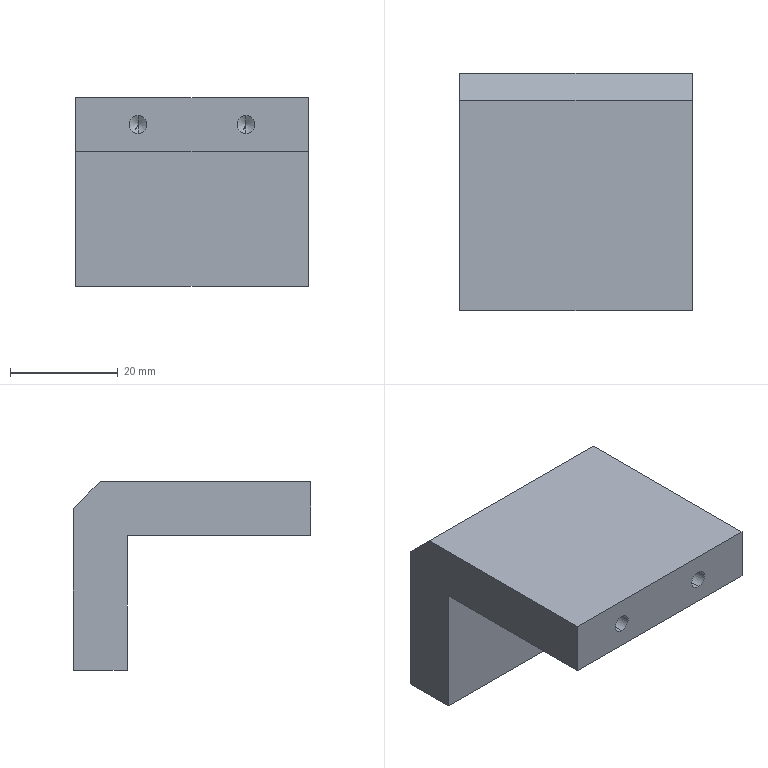Part | SolidWorks | features HoleWzd 2, Chamfer 1, Extrusion 1, ICE 1 | 1 solid | 25 faces | box 43 x 44 x 35 mm | volume 28591 mm3 | plane 9 | cylinder 8 | cone 8 | commonest cylinder face diameters 3.3 x8
STEP:
#1=CARTESIAN_POINT('',(-10.,-6.5,14.15));
#2=VERTEX_POINT('',#1);
#3=CARTESIAN_POINT('',(-10.,-6.5,10.85));
#4=VERTEX_POINT('',#3);
#5=CARTESIAN_POINT('',(-10.,-6.5,12.5));
#6=DIRECTION('',(0.,-1.,0.));
#7=DIRECTION('',(0.,0.,-1.));
#8=AXIS2_PLACEMENT_3D('',#5,#6,#7);
#9=CIRCLE('',#8,1.65);
#10=EDGE_CURVE('',#2,#4,#9,.T.);
#11=ORIENTED_EDGE('',*,*,#10,.F.);
#12=CARTESIAN_POINT('',(-10.,-22.,14.15));
#13=VERTEX_POINT('',#12);
#14=CARTESIAN_POINT('',(-10.,-22.,14.15));
#15=DIRECTION('',(0.,-1.,0.));
#16=VECTOR('',#15,1000.);
#17=LINE('',#14,#16);
#18=EDGE_CURVE('',#2,#13,#17,.T.);
#19=ORIENTED_EDGE('',*,*,#18,.T.);
#20=CARTESIAN_POINT('',(-10.,-22.,10.85));
#21=VERTEX_POINT('',#20);
#22=CARTESIAN_POINT('',(-10.,-22.,12.5));
#23=DIRECTION('',(0.,-1.,0.));
#24=DIRECTION('',(0.,0.,-1.));
#25=AXIS2_PLACEMENT_3D('',#22,#23,#24);
#26=CIRCLE('',#25,1.65);
#27=EDGE_CURVE('',#13,#21,#26,.T.);
#28=ORIENTED_EDGE('',*,*,#27,.T.);
#29=CARTESIAN_POINT('',(-10.,-22.,10.85));
#30=DIRECTION('',(0.,-1.,0.));
#31=VECTOR('',#30,1000.);
#32=LINE('',#29,#31);
#33=EDGE_CURVE('',#4,#21,#32,.T.);
#34=ORIENTED_EDGE('',*,*,#33,.F.);
#35=EDGE_LOOP('',(#11,#19,#28,#34));
#36=FACE_OUTER_BOUND('',#35,.T.);
#37=CARTESIAN_POINT('',(-10.,-22.,12.5));
#38=DIRECTION('',(0.,-1.,0.));
#39=DIRECTION('',(0.,0.,-1.));
#40=AXIS2_PLACEMENT_3D('',#37,#38,#39);
#41=CYLINDRICAL_SURFACE('',#40,1.65);
#42=ADVANCED_FACE('',(#36),#41,.F.);
#43=CARTESIAN_POINT('',(-10.,-5.509,12.5));
#44=VERTEX_POINT('',#43);
#45=CARTESIAN_POINT('',(-10.,-6.5,10.85));
#46=DIRECTION('',(0.,-0.515,-0.8572));
#47=VECTOR('',#46,1000.);
#48=LINE('',#45,#47);
#49=EDGE_CURVE('',#44,#4,#48,.T.);
#50=ORIENTED_EDGE('',*,*,#49,.F.);
#51=CARTESIAN_POINT('',(-10.,-6.5,14.15));
#52=DIRECTION('',(0.,-0.515,0.8572));
#53=VECTOR('',#52,1000.);
#54=LINE('',#51,#53);
#55=EDGE_CURVE('',#44,#2,#54,.T.);
#56=ORIENTED_EDGE('',*,*,#55,.T.);
#57=ORIENTED_EDGE('',*,*,#10,.T.);
#58=EDGE_LOOP('',(#50,#56,#57));
#59=FACE_OUTER_BOUND('',#58,.T.);
#60=CARTESIAN_POINT('',(-10.,-6.5,12.5));
#61=DIRECTION('',(0.,-1.,0.));
#62=DIRECTION('',(0.,0.,-1.));
#63=AXIS2_PLACEMENT_3D('',#60,#61,#62);
#64=CONICAL_SURFACE('',#63,1.65,1.03);
#65=ADVANCED_FACE('',(#59),#64,.F.);
#66=CARTESIAN_POINT('',(10.,-6.5,14.15));
#67=VERTEX_POINT('',#66);
#68=CARTESIAN_POINT('',(10.,-6.5,10.85));
#69=VERTEX_POINT('',#68);
#70=CARTESIAN_POINT('',(10.,-6.5,12.5));
#71=DIRECTION('',(0.,-1.,0.));
#72=DIRECTION('',(0.,0.,-1.));
#73=AXIS2_PLACEMENT_3D('',#70,#71,#72);
#74=CIRCLE('',#73,1.65);
#75=EDGE_CURVE('',#67,#69,#74,.T.);
#76=ORIENTED_EDGE('',*,*,#75,.F.);
#77=CARTESIAN_POINT('',(10.,-22.,14.15));
#78=VERTEX_POINT('',#77);
#79=CARTESIAN_POINT('',(10.,-22.,14.15));
#80=DIRECTION('',(0.,-1.,0.));
#81=VECTOR('',#80,1000.);
#82=LINE('',#79,#81);
#83=EDGE_CURVE('',#67,#78,#82,.T.);
#84=ORIENTED_EDGE('',*,*,#83,.T.);
#85=CARTESIAN_POINT('',(10.,-22.,10.85));
#86=VERTEX_POINT('',#85);
#87=CARTESIAN_POINT('',(10.,-22.,12.5));
#88=DIRECTION('',(0.,-1.,0.));
#89=DIRECTION('',(0.,0.,-1.));
#90=AXIS2_PLACEMENT_3D('',#87,#88,#89);
#91=CIRCLE('',#90,1.65);
#92=EDGE_CURVE('',#78,#86,#91,.T.);
#93=ORIENTED_EDGE('',*,*,#92,.T.);
#94=CARTESIAN_POINT('',(10.,-22.,10.85));
#95=DIRECTION('',(0.,-1.,0.));
#96=VECTOR('',#95,1000.);
#97=LINE('',#94,#96);
#98=EDGE_CURVE('',#69,#86,#97,.T.);
#99=ORIENTED_EDGE('',*,*,#98,.F.);
#100=EDGE_LOOP('',(#76,#84,#93,#99));
#101=FACE_OUTER_BOUND('',#100,.T.);
#102=CARTESIAN_POINT('',(10.,-22.,12.5));
#103=DIRECTION('',(0.,-1.,0.));
#104=DIRECTION('',(0.,0.,-1.));
#105=AXIS2_PLACEMENT_3D('',#102,#103,#104);
#106=CYLINDRICAL_SURFACE('',#105,1.65);
#107=ADVANCED_FACE('',(#101),#106,.F.);
#108=CARTESIAN_POINT('',(10.,-5.509,12.5));
#109=VERTEX_POINT('',#108);
#110=CARTESIAN_POINT('',(10.,-6.5,10.85));
#111=DIRECTION('',(0.,-0.515,-0.8572));
#112=VECTOR('',#111,1000.);
#113=LINE('',#110,#112);
#114=EDGE_CURVE('',#109,#69,#113,.T.);
#115=ORIENTED_EDGE('',*,*,#114,.F.);
#116=CARTESIAN_POINT('',(10.,-6.5,14.15));
#117=DIRECTION('',(0.,-0.515,0.8572));
#118=VECTOR('',#117,1000.);
#119=LINE('',#116,#118);
#120=EDGE_CURVE('',#109,#67,#119,.T.);
#121=ORIENTED_EDGE('',*,*,#120,.T.);
#122=ORIENTED_EDGE('',*,*,#75,.T.);
#123=EDGE_LOOP('',(#115,#121,#122));
#124=FACE_OUTER_BOUND('',#123,.T.);
#125=CARTESIAN_POINT('',(10.,-6.5,12.5));
#126=DIRECTION('',(0.,-1.,0.));
#127=DIRECTION('',(0.,0.,-1.));
#128=AXIS2_PLACEMENT_3D('',#125,#126,#127);
#129=CONICAL_SURFACE('',#128,1.65,1.03);
#130=ADVANCED_FACE('',(#124),#129,.F.);
#131=CARTESIAN_POINT('',(16.65,17.,-2.));
#132=VERTEX_POINT('',#131);
#133=CARTESIAN_POINT('',(13.35,17.,-2.));
#134=VERTEX_POINT('',#133);
#135=CARTESIAN_POINT('',(15.,17.,-2.));
#136=DIRECTION('',(0.,0.,-1.));
#137=DIRECTION('',(-1.,0.,0.));
#138=AXIS2_PLACEMENT_3D('',#135,#136,#137);
#139=CIRCLE('',#138,1.65);
#140=EDGE_CURVE('',#132,#134,#139,.T.);
#141=ORIENTED_EDGE('',*,*,#140,.F.);
#142=CARTESIAN_POINT('',(16.65,17.,-17.5));
#143=VERTEX_POINT('',#142);
#144=CARTESIAN_POINT('',(16.65,17.,-17.5));
#145=DIRECTION('',(0.,0.,-1.));
#146=VECTOR('',#145,1000.);
#147=LINE('',#144,#146);
#148=EDGE_CURVE('',#132,#143,#147,.T.);
#149=ORIENTED_EDGE('',*,*,#148,.T.);
#150=CARTESIAN_POINT('',(13.35,17.,-17.5));
#151=VERTEX_POINT('',#150);
#152=CARTESIAN_POINT('',(15.,17.,-17.5));
#153=DIRECTION('',(0.,0.,-1.));
#154=DIRECTION('',(-1.,0.,0.));
#155=AXIS2_PLACEMENT_3D('',#152,#153,#154);
#156=CIRCLE('',#155,1.65);
#157=EDGE_CURVE('',#143,#151,#156,.T.);
#158=ORIENTED_EDGE('',*,*,#157,.T.);
#159=CARTESIAN_POINT('',(13.35,17.,-17.5));
#160=DIRECTION('',(0.,0.,-1.));
#161=VECTOR('',#160,1000.);
#162=LINE('',#159,#161);
#163=EDGE_CURVE('',#134,#151,#162,.T.);
#164=ORIENTED_EDGE('',*,*,#163,.F.);
#165=EDGE_LOOP('',(#141,#149,#158,#164));
#166=FACE_OUTER_BOUND('',#165,.T.);
#167=CARTESIAN_POINT('',(15.,17.,-17.5));
#168=DIRECTION('',(0.,0.,-1.));
#169=DIRECTION('',(-1.,0.,0.));
#170=AXIS2_PLACEMENT_3D('',#167,#168,#169);
#171=CYLINDRICAL_SURFACE('',#170,1.65);
#172=ADVANCED_FACE('',(#166),#171,.F.);
#173=CARTESIAN_POINT('',(15.,17.,-1.009));
#174=VERTEX_POINT('',#173);
#175=CARTESIAN_POINT('',(13.35,17.,-2.));
#176=DIRECTION('',(-0.8572,0.,-0.515));
#177=VECTOR('',#176,1000.);
#178=LINE('',#175,#177);
#179=EDGE_CURVE('',#174,#134,#178,.T.);
#180=ORIENTED_EDGE('',*,*,#179,.F.);
#181=CARTESIAN_POINT('',(16.65,17.,-2.));
#182=DIRECTION('',(0.8572,0.,-0.515));
#183=VECTOR('',#182,1000.);
#184=LINE('',#181,#183);
#185=EDGE_CURVE('',#174,#132,#184,.T.);
#186=ORIENTED_EDGE('',*,*,#185,.T.);
#187=ORIENTED_EDGE('',*,*,#140,.T.);
#188=EDGE_LOOP('',(#180,#186,#187));
#189=FACE_OUTER_BOUND('',#188,.T.);
#190=CARTESIAN_POINT('',(15.,17.,-2.));
#191=DIRECTION('',(0.,0.,-1.));
#192=DIRECTION('',(-1.,0.,0.));
#193=AXIS2_PLACEMENT_3D('',#190,#191,#192);
#194=CONICAL_SURFACE('',#193,1.65,1.03);
#195=ADVANCED_FACE('',(#189),#194,.F.);
#196=CARTESIAN_POINT('',(-13.35,17.,-2.));
#197=VERTEX_POINT('',#196);
#198=CARTESIAN_POINT('',(-16.65,17.,-2.));
#199=VERTEX_POINT('',#198);
#200=CARTESIAN_POINT('',(-15.,17.,-2.));
#201=DIRECTION('',(0.,0.,-1.));
#202=DIRECTION('',(-1.,0.,0.));
#203=AXIS2_PLACEMENT_3D('',#200,#201,#202);
#204=CIRCLE('',#203,1.65);
#205=EDGE_CURVE('',#197,#199,#204,.T.);
#206=ORIENTED_EDGE('',*,*,#205,.F.);
#207=CARTESIAN_POINT('',(-13.35,17.,-17.5));
#208=VERTEX_POINT('',#207);
#209=CARTESIAN_POINT('',(-13.35,17.,-17.5));
#210=DIRECTION('',(0.,0.,-1.));
#211=VECTOR('',#210,1000.);
#212=LINE('',#209,#211);
#213=EDGE_CURVE('',#197,#208,#212,.T.);
#214=ORIENTED_EDGE('',*,*,#213,.T.);
#215=CARTESIAN_POINT('',(-16.65,17.,-17.5));
#216=VERTEX_POINT('',#215);
#217=CARTESIAN_POINT('',(-15.,17.,-17.5));
#218=DIRECTION('',(0.,0.,-1.));
#219=DIRECTION('',(-1.,0.,0.));
#220=AXIS2_PLACEMENT_3D('',#217,#218,#219);
#221=CIRCLE('',#220,1.65);
#222=EDGE_CURVE('',#208,#216,#221,.T.);
#223=ORIENTED_EDGE('',*,*,#222,.T.);
#224=CARTESIAN_POINT('',(-16.65,17.,-17.5));
#225=DIRECTION('',(0.,0.,-1.));
#226=VECTOR('',#225,1000.);
#227=LINE('',#224,#226);
#228=EDGE_CURVE('',#199,#216,#227,.T.);
#229=ORIENTED_EDGE('',*,*,#228,.F.);
#230=EDGE_LOOP('',(#206,#214,#223,#229));
#231=FACE_OUTER_BOUND('',#230,.T.);
#232=CARTESIAN_POINT('',(-15.,17.,-17.5));
#233=DIRECTION('',(0.,0.,-1.));
#234=DIRECTION('',(-1.,0.,0.));
#235=AXIS2_PLACEMENT_3D('',#232,#233,#234);
#236=CYLINDRICAL_SURFACE('',#235,1.65);
#237=ADVANCED_FACE('',(#231),#236,.F.);
#238=CARTESIAN_POINT('',(-15.,17.,-1.009));
#239=VERTEX_POINT('',#238);
#240=CARTESIAN_POINT('',(-16.65,17.,-2.));
#241=DIRECTION('',(-0.8572,0.,-0.515));
#242=VECTOR('',#241,1000.);
#243=LINE('',#240,#242);
#244=EDGE_CURVE('',#239,#199,#243,.T.);
#245=ORIENTED_EDGE('',*,*,#244,.F.);
#246=CARTESIAN_POINT('',(-13.35,17.,-2.));
#247=DIRECTION('',(0.8572,0.,-0.515));
#248=VECTOR('',#247,1000.);
#249=LINE('',#246,#248);
#250=EDGE_CURVE('',#239,#197,#249,.T.);
#251=ORIENTED_EDGE('',*,*,#250,.T.);
#252=ORIENTED_EDGE('',*,*,#205,.T.);
#253=EDGE_LOOP('',(#245,#251,#252));
#254=FACE_OUTER_BOUND('',#253,.T.);
#255=CARTESIAN_POINT('',(-15.,17.,-2.));
#256=DIRECTION('',(0.,0.,-1.));
#257=DIRECTION('',(-1.,0.,0.));
#258=AXIS2_PLACEMENT_3D('',#255,#256,#257);
#259=CONICAL_SURFACE('',#258,1.65,1.03);
#260=ADVANCED_FACE('',(#254),#259,.F.);
#261=CARTESIAN_POINT('',(21.5,22.,12.5));
#262=VERTEX_POINT('',#261);
#263=CARTESIAN_POINT('',(21.5,22.,-17.5));
#264=VERTEX_POINT('',#263);
#265=CARTESIAN_POINT('',(21.5,22.,17.5));
#266=DIRECTION('',(0.,0.,-1.));
#267=VECTOR('',#266,1000.);
#268=LINE('',#265,#267);
#269=EDGE_CURVE('',#262,#264,#268,.T.);
#270=ORIENTED_EDGE('',*,*,#269,.F.);
#271=CARTESIAN_POINT('',(21.5,17.,17.5));
#272=VERTEX_POINT('',#271);
#273=CARTESIAN_POINT('',(21.5,17.,17.5));
#274=DIRECTION('',(0.,-0.7071,0.7071));
#275=VECTOR('',#274,1000.);
#276=LINE('',#273,#275);
#277=EDGE_CURVE('',#262,#272,#276,.T.);
#278=ORIENTED_EDGE('',*,*,#277,.T.);
#279=CARTESIAN_POINT('',(21.5,-22.,17.5));
#280=VERTEX_POINT('',#279);
#281=CARTESIAN_POINT('',(21.5,22.,17.5));
#282=DIRECTION('',(0.,1.,0.));
#283=VECTOR('',#282,1000.);
#284=LINE('',#281,#283);
#285=EDGE_CURVE('',#280,#272,#284,.T.);
#286=ORIENTED_EDGE('',*,*,#285,.F.);
#287=CARTESIAN_POINT('',(21.5,-22.,7.5));
#288=VERTEX_POINT('',#287);
#289=CARTESIAN_POINT('',(21.5,-22.,17.5));
#290=DIRECTION('',(0.,0.,-1.));
#291=VECTOR('',#290,1000.);
#292=LINE('',#289,#291);
#293=EDGE_CURVE('',#280,#288,#292,.T.);
#294=ORIENTED_EDGE('',*,*,#293,.T.);
#295=CARTESIAN_POINT('',(21.5,12.,7.5));
#296=VERTEX_POINT('',#295);
#297=CARTESIAN_POINT('',(21.5,-56.,7.5));
#298=DIRECTION('',(0.,-1.,0.));
#299=VECTOR('',#298,1000.);
#300=LINE('',#297,#299);
#301=EDGE_CURVE('',#296,#288,#300,.T.);
#302=ORIENTED_EDGE('',*,*,#301,.F.);
#303=CARTESIAN_POINT('',(21.5,12.,-17.5));
#304=VERTEX_POINT('',#303);
#305=CARTESIAN_POINT('',(21.5,12.,-42.5));
#306=DIRECTION('',(0.,0.,1.));
#307=VECTOR('',#306,1000.);
#308=LINE('',#305,#307);
#309=EDGE_CURVE('',#304,#296,#308,.T.);
#310=ORIENTED_EDGE('',*,*,#309,.F.);
#311=CARTESIAN_POINT('',(21.5,22.,-17.5));
#312=DIRECTION('',(0.,1.,0.));
#313=VECTOR('',#312,1000.);
#314=LINE('',#311,#313);
#315=EDGE_CURVE('',#304,#264,#314,.T.);
#316=ORIENTED_EDGE('',*,*,#315,.T.);
#317=EDGE_LOOP('',(#270,#278,#286,#294,#302,#310,#316));
#318=FACE_OUTER_BOUND('',#317,.T.);
#319=CARTESIAN_POINT('',(21.5,22.,17.5));
#320=DIRECTION('',(-1.,0.,0.));
#321=DIRECTION('',(0.,-1.,0.));
#322=AXIS2_PLACEMENT_3D('',#319,#320,#321);
#323=PLANE('',#322);
#324=ADVANCED_FACE('',(#318),#323,.F.);
#325=CARTESIAN_POINT('',(-21.5,22.,12.5));
#326=VERTEX_POINT('',#325);
#327=CARTESIAN_POINT('',(-21.5,22.,-17.5));
#328=VERTEX_POINT('',#327);
#329=CARTESIAN_POINT('',(-21.5,22.,17.5));
#330=DIRECTION('',(0.,0.,-1.));
#331=VECTOR('',#330,1000.);
#332=LINE('',#329,#331);
#333=EDGE_CURVE('',#326,#328,#332,.T.);
#334=ORIENTED_EDGE('',*,*,#333,.F.);
#335=CARTESIAN_POINT('',(21.5,22.,12.5));
#336=DIRECTION('',(1.,0.,0.));
#337=VECTOR('',#336,1000.);
#338=LINE('',#335,#337);
#339=EDGE_CURVE('',#326,#262,#338,.T.);
#340=ORIENTED_EDGE('',*,*,#339,.T.);
#341=ORIENTED_EDGE('',*,*,#269,.T.);
#342=CARTESIAN_POINT('',(-21.5,22.,-17.5));
#343=DIRECTION('',(-1.,0.,0.));
#344=VECTOR('',#343,1000.);
#345=LINE('',#342,#344);
#346=EDGE_CURVE('',#264,#328,#345,.T.);
#347=ORIENTED_EDGE('',*,*,#346,.T.);
#348=EDGE_LOOP('',(#334,#340,#341,#347));
#349=FACE_OUTER_BOUND('',#348,.T.);
#350=CARTESIAN_POINT('',(-21.5,22.,17.5));
#351=DIRECTION('',(0.,-1.,0.));
#352=DIRECTION('',(0.,0.,-1.));
#353=AXIS2_PLACEMENT_3D('',#350,#351,#352);
#354=PLANE('',#353);
#355=ADVANCED_FACE('',(#349),#354,.F.);
#356=CARTESIAN_POINT('',(-21.5,17.,17.5));
#357=VERTEX_POINT('',#356);
#358=CARTESIAN_POINT('',(-21.5,-22.,17.5));
#359=VERTEX_POINT('',#358);
#360=CARTESIAN_POINT('',(-21.5,22.,17.5));
#361=DIRECTION('',(0.,-1.,0.));
#362=VECTOR('',#361,1000.);
#363=LINE('',#360,#362);
#364=EDGE_CURVE('',#357,#359,#363,.T.);
#365=ORIENTED_EDGE('',*,*,#364,.F.);
#366=CARTESIAN_POINT('',(-21.5,17.,17.5));
#367=DIRECTION('',(0.,0.7071,-0.7071));
#368=VECTOR('',#367,1000.);
#369=LINE('',#366,#368);
#370=EDGE_CURVE('',#357,#326,#369,.T.);
#371=ORIENTED_EDGE('',*,*,#370,.T.);
#372=ORIENTED_EDGE('',*,*,#333,.T.);
#373=CARTESIAN_POINT('',(-21.5,12.,-17.5));
#374=VERTEX_POINT('',#373);
#375=CARTESIAN_POINT('',(-21.5,22.,-17.5));
#376=DIRECTION('',(0.,-1.,0.));
#377=VECTOR('',#376,1000.);
#378=LINE('',#375,#377);
#379=EDGE_CURVE('',#328,#374,#378,.T.);
#380=ORIENTED_EDGE('',*,*,#379,.T.);
#381=CARTESIAN_POINT('',(-21.5,12.,7.5));
#382=VERTEX_POINT('',#381);
#383=CARTESIAN_POINT('',(-21.5,12.,-42.5));
#384=DIRECTION('',(0.,0.,1.));
#385=VECTOR('',#384,1000.);
#386=LINE('',#383,#385);
#387=EDGE_CURVE('',#374,#382,#386,.T.);
#388=ORIENTED_EDGE('',*,*,#387,.T.);
#389=CARTESIAN_POINT('',(-21.5,-22.,7.5));
#390=VERTEX_POINT('',#389);
#391=CARTESIAN_POINT('',(-21.5,-56.,7.5));
#392=DIRECTION('',(0.,-1.,0.));
#393=VECTOR('',#392,1000.);
#394=LINE('',#391,#393);
#395=EDGE_CURVE('',#382,#390,#394,.T.);
#396=ORIENTED_EDGE('',*,*,#395,.T.);
#397=CARTESIAN_POINT('',(-21.5,-22.,17.5));
#398=DIRECTION('',(0.,0.,-1.));
#399=VECTOR('',#398,1000.);
#400=LINE('',#397,#399);
#401=EDGE_CURVE('',#359,#390,#400,.T.);
#402=ORIENTED_EDGE('',*,*,#401,.F.);
#403=EDGE_LOOP('',(#365,#371,#372,#380,#388,#396,#402));
#404=FACE_OUTER_BOUND('',#403,.T.);
#405=CARTESIAN_POINT('',(-21.5,22.,17.5));
#406=DIRECTION('',(1.,0.,0.));
#407=DIRECTION('',(0.,1.,0.));
#408=AXIS2_PLACEMENT_3D('',#405,#406,#407);
#409=PLANE('',#408);
#410=ADVANCED_FACE('',(#404),#409,.F.);
#411=CARTESIAN_POINT('',(-10.,-22.,12.5));
#412=DIRECTION('',(0.,-1.,0.));
#413=DIRECTION('',(0.,0.,-1.));
#414=AXIS2_PLACEMENT_3D('',#411,#412,#413);
#415=CIRCLE('',#414,1.65);
#416=EDGE_CURVE('',#21,#13,#415,.T.);
#417=ORIENTED_EDGE('',*,*,#416,.F.);
#418=ORIENTED_EDGE('',*,*,#27,.F.);
#419=EDGE_LOOP('',(#417,#418));
#420=FACE_BOUND('',#419,.T.);
#421=CARTESIAN_POINT('',(10.,-22.,12.5));
#422=DIRECTION('',(0.,-1.,0.));
#423=DIRECTION('',(0.,0.,-1.));
#424=AXIS2_PLACEMENT_3D('',#421,#422,#423);
#425=CIRCLE('',#424,1.65);
#426=EDGE_CURVE('',#86,#78,#425,.T.);
#427=ORIENTED_EDGE('',*,*,#426,.F.);
#428=ORIENTED_EDGE('',*,*,#92,.F.);
#429=EDGE_LOOP('',(#427,#428));
#430=FACE_BOUND('',#429,.T.);
#431=ORIENTED_EDGE('',*,*,#401,.T.);
#432=CARTESIAN_POINT('',(-21.5,-22.,7.5));
#433=DIRECTION('',(1.,0.,0.));
#434=VECTOR('',#433,1000.);
#435=LINE('',#432,#434);
#436=EDGE_CURVE('',#390,#288,#435,.T.);
#437=ORIENTED_EDGE('',*,*,#436,.T.);
#438=ORIENTED_EDGE('',*,*,#293,.F.);
#439=CARTESIAN_POINT('',(-21.5,-22.,17.5));
#440=DIRECTION('',(1.,0.,0.));
#441=VECTOR('',#440,1000.);
#442=LINE('',#439,#441);
#443=EDGE_CURVE('',#359,#280,#442,.T.);
#444=ORIENTED_EDGE('',*,*,#443,.F.);
#445=EDGE_LOOP('',(#431,#437,#438,#444));
#446=FACE_OUTER_BOUND('',#445,.T.);
#447=CARTESIAN_POINT('',(-21.5,-22.,17.5));
#448=DIRECTION('',(0.,1.,0.));
#449=DIRECTION('',(0.,0.,1.));
#450=AXIS2_PLACEMENT_3D('',#447,#448,#449);
#451=PLANE('',#450);
#452=ADVANCED_FACE('',(#420,#430,#446),#451,.F.);
#453=ORIENTED_EDGE('',*,*,#285,.T.);
#454=CARTESIAN_POINT('',(-21.5,17.,17.5));
#455=DIRECTION('',(-1.,0.,0.));
#456=VECTOR('',#455,1000.);
#457=LINE('',#454,#456);
#458=EDGE_CURVE('',#272,#357,#457,.T.);
#459=ORIENTED_EDGE('',*,*,#458,.T.);
#460=ORIENTED_EDGE('',*,*,#364,.T.);
#461=ORIENTED_EDGE('',*,*,#443,.T.);
#462=EDGE_LOOP('',(#453,#459,#460,#461));
#463=FACE_OUTER_BOUND('',#462,.T.);
#464=CARTESIAN_POINT('',(0.,0.,17.5));
#465=DIRECTION('',(0.,0.,1.));
#466=DIRECTION('',(1.,0.,0.));
#467=AXIS2_PLACEMENT_3D('',#464,#465,#466);
#468=PLANE('',#467);
#469=ADVANCED_FACE('',(#463),#468,.T.);
#470=CARTESIAN_POINT('',(15.,17.,-17.5));
#471=DIRECTION('',(0.,0.,-1.));
#472=DIRECTION('',(-1.,0.,0.));
#473=AXIS2_PLACEMENT_3D('',#470,#471,#472);
#474=CIRCLE('',#473,1.65);
#475=EDGE_CURVE('',#151,#143,#474,.T.);
#476=ORIENTED_EDGE('',*,*,#475,.F.);
#477=ORIENTED_EDGE('',*,*,#157,.F.);
#478=EDGE_LOOP('',(#476,#477));
#479=FACE_BOUND('',#478,.T.);
#480=CARTESIAN_POINT('',(-15.,17.,-17.5));
#481=DIRECTION('',(0.,0.,-1.));
#482=DIRECTION('',(-1.,0.,0.));
#483=AXIS2_PLACEMENT_3D('',#480,#481,#482);
#484=CIRCLE('',#483,1.65);
#485=EDGE_CURVE('',#216,#208,#484,.T.);
#486=ORIENTED_EDGE('',*,*,#485,.F.);
#487=ORIENTED_EDGE('',*,*,#222,.F.);
#488=EDGE_LOOP('',(#486,#487));
#489=FACE_BOUND('',#488,.T.);
#490=ORIENTED_EDGE('',*,*,#315,.F.);
#491=CARTESIAN_POINT('',(0.,12.,-17.5));
#492=DIRECTION('',(-1.,0.,0.));
#493=VECTOR('',#492,1000.);
#494=LINE('',#491,#493);
#495=EDGE_CURVE('',#304,#374,#494,.T.);
#496=ORIENTED_EDGE('',*,*,#495,.T.);
#497=ORIENTED_EDGE('',*,*,#379,.F.);
#498=ORIENTED_EDGE('',*,*,#346,.F.);
#499=EDGE_LOOP('',(#490,#496,#497,#498));
#500=FACE_OUTER_BOUND('',#499,.T.);
#501=CARTESIAN_POINT('',(0.,0.,-17.5));
#502=DIRECTION('',(0.,0.,1.));
#503=DIRECTION('',(1.,0.,0.));
#504=AXIS2_PLACEMENT_3D('',#501,#502,#503);
#505=PLANE('',#504);
#506=ADVANCED_FACE('',(#479,#489,#500),#505,.F.);
#507=ORIENTED_EDGE('',*,*,#395,.F.);
#508=CARTESIAN_POINT('',(-21.5,12.,7.5));
#509=DIRECTION('',(1.,0.,0.));
#510=VECTOR('',#509,1000.);
#511=LINE('',#508,#510);
#512=EDGE_CURVE('',#382,#296,#511,.T.);
#513=ORIENTED_EDGE('',*,*,#512,.T.);
#514=ORIENTED_EDGE('',*,*,#301,.T.);
#515=ORIENTED_EDGE('',*,*,#436,.F.);
#516=EDGE_LOOP('',(#507,#513,#514,#515));
#517=FACE_OUTER_BOUND('',#516,.T.);
#518=CARTESIAN_POINT('',(-21.5,-56.,7.5));
#519=DIRECTION('',(0.,0.,1.));
#520=DIRECTION('',(1.,0.,0.));
#521=AXIS2_PLACEMENT_3D('',#518,#519,#520);
#522=PLANE('',#521);
#523=ADVANCED_FACE('',(#517),#522,.F.);
#524=ORIENTED_EDGE('',*,*,#309,.T.);
#525=ORIENTED_EDGE('',*,*,#512,.F.);
#526=ORIENTED_EDGE('',*,*,#387,.F.);
#527=ORIENTED_EDGE('',*,*,#495,.F.);
#528=EDGE_LOOP('',(#524,#525,#526,#527));
#529=FACE_OUTER_BOUND('',#528,.T.);
#530=CARTESIAN_POINT('',(-21.5,12.,-42.5));
#531=DIRECTION('',(0.,1.,0.));
#532=DIRECTION('',(-1.,0.,0.));
#533=AXIS2_PLACEMENT_3D('',#530,#531,#532);
#534=PLANE('',#533);
#535=ADVANCED_FACE('',(#529),#534,.F.);
#536=ORIENTED_EDGE('',*,*,#250,.F.);
#537=ORIENTED_EDGE('',*,*,#244,.T.);
#538=CARTESIAN_POINT('',(-15.,17.,-2.));
#539=DIRECTION('',(0.,0.,-1.));
#540=DIRECTION('',(-1.,0.,0.));
#541=AXIS2_PLACEMENT_3D('',#538,#539,#540);
#542=CIRCLE('',#541,1.65);
#543=EDGE_CURVE('',#199,#197,#542,.T.);
#544=ORIENTED_EDGE('',*,*,#543,.T.);
#545=EDGE_LOOP('',(#536,#537,#544));
#546=FACE_OUTER_BOUND('',#545,.T.);
#547=CARTESIAN_POINT('',(-15.,17.,-2.));
#548=DIRECTION('',(0.,0.,-1.));
#549=DIRECTION('',(-1.,0.,0.));
#550=AXIS2_PLACEMENT_3D('',#547,#548,#549);
#551=CONICAL_SURFACE('',#550,1.65,1.03);
#552=ADVANCED_FACE('',(#546),#551,.F.);
#553=ORIENTED_EDGE('',*,*,#213,.F.);
#554=ORIENTED_EDGE('',*,*,#543,.F.);
#555=ORIENTED_EDGE('',*,*,#228,.T.);
#556=ORIENTED_EDGE('',*,*,#485,.T.);
#557=EDGE_LOOP('',(#553,#554,#555,#556));
#558=FACE_OUTER_BOUND('',#557,.T.);
#559=CARTESIAN_POINT('',(-15.,17.,-17.5));
#560=DIRECTION('',(0.,0.,-1.));
#561=DIRECTION('',(-1.,0.,0.));
#562=AXIS2_PLACEMENT_3D('',#559,#560,#561);
#563=CYLINDRICAL_SURFACE('',#562,1.65);
#564=ADVANCED_FACE('',(#558),#563,.F.);
#565=ORIENTED_EDGE('',*,*,#185,.F.);
#566=ORIENTED_EDGE('',*,*,#179,.T.);
#567=CARTESIAN_POINT('',(15.,17.,-2.));
#568=DIRECTION('',(0.,0.,-1.));
#569=DIRECTION('',(-1.,0.,0.));
#570=AXIS2_PLACEMENT_3D('',#567,#568,#569);
#571=CIRCLE('',#570,1.65);
#572=EDGE_CURVE('',#134,#132,#571,.T.);
#573=ORIENTED_EDGE('',*,*,#572,.T.);
#574=EDGE_LOOP('',(#565,#566,#573));
#575=FACE_OUTER_BOUND('',#574,.T.);
#576=CARTESIAN_POINT('',(15.,17.,-2.));
#577=DIRECTION('',(0.,0.,-1.));
#578=DIRECTION('',(-1.,0.,0.));
#579=AXIS2_PLACEMENT_3D('',#576,#577,#578);
#580=CONICAL_SURFACE('',#579,1.65,1.03);
#581=ADVANCED_FACE('',(#575),#580,.F.);
#582=ORIENTED_EDGE('',*,*,#148,.F.);
#583=ORIENTED_EDGE('',*,*,#572,.F.);
#584=ORIENTED_EDGE('',*,*,#163,.T.);
#585=ORIENTED_EDGE('',*,*,#475,.T.);
#586=EDGE_LOOP('',(#582,#583,#584,#585));
#587=FACE_OUTER_BOUND('',#586,.T.);
#588=CARTESIAN_POINT('',(15.,17.,-17.5));
#589=DIRECTION('',(0.,0.,-1.));
#590=DIRECTION('',(-1.,0.,0.));
#591=AXIS2_PLACEMENT_3D('',#588,#589,#590);
#592=CYLINDRICAL_SURFACE('',#591,1.65);
#593=ADVANCED_FACE('',(#587),#592,.F.);
#594=ORIENTED_EDGE('',*,*,#277,.F.);
#595=ORIENTED_EDGE('',*,*,#339,.F.);
#596=ORIENTED_EDGE('',*,*,#370,.F.);
#597=ORIENTED_EDGE('',*,*,#458,.F.);
#598=EDGE_LOOP('',(#594,#595,#596,#597));
#599=FACE_OUTER_BOUND('',#598,.T.);
#600=CARTESIAN_POINT('',(0.,17.,17.5));
#601=DIRECTION('',(0.,0.7071,0.7071));
#602=DIRECTION('',(1.,0.,0.));
#603=AXIS2_PLACEMENT_3D('',#600,#601,#602);
#604=PLANE('',#603);
#605=ADVANCED_FACE('',(#599),#604,.T.);
#606=ORIENTED_EDGE('',*,*,#120,.F.);
#607=ORIENTED_EDGE('',*,*,#114,.T.);
#608=CARTESIAN_POINT('',(10.,-6.5,12.5));
#609=DIRECTION('',(0.,-1.,0.));
#610=DIRECTION('',(0.,0.,-1.));
#611=AXIS2_PLACEMENT_3D('',#608,#609,#610);
#612=CIRCLE('',#611,1.65);
#613=EDGE_CURVE('',#69,#67,#612,.T.);
#614=ORIENTED_EDGE('',*,*,#613,.T.);
#615=EDGE_LOOP('',(#606,#607,#614));
#616=FACE_OUTER_BOUND('',#615,.T.);
#617=CARTESIAN_POINT('',(10.,-6.5,12.5));
#618=DIRECTION('',(0.,-1.,0.));
#619=DIRECTION('',(0.,0.,-1.));
#620=AXIS2_PLACEMENT_3D('',#617,#618,#619);
#621=CONICAL_SURFACE('',#620,1.65,1.03);
#622=ADVANCED_FACE('',(#616),#621,.F.);
#623=ORIENTED_EDGE('',*,*,#83,.F.);
#624=ORIENTED_EDGE('',*,*,#613,.F.);
#625=ORIENTED_EDGE('',*,*,#98,.T.);
#626=ORIENTED_EDGE('',*,*,#426,.T.);
#627=EDGE_LOOP('',(#623,#624,#625,#626));
#628=FACE_OUTER_BOUND('',#627,.T.);
#629=CARTESIAN_POINT('',(10.,-22.,12.5));
#630=DIRECTION('',(0.,-1.,0.));
#631=DIRECTION('',(0.,0.,-1.));
#632=AXIS2_PLACEMENT_3D('',#629,#630,#631);
#633=CYLINDRICAL_SURFACE('',#632,1.65);
#634=ADVANCED_FACE('',(#628),#633,.F.);
#635=ORIENTED_EDGE('',*,*,#55,.F.);
#636=ORIENTED_EDGE('',*,*,#49,.T.);
#637=CARTESIAN_POINT('',(-10.,-6.5,12.5));
#638=DIRECTION('',(0.,-1.,0.));
#639=DIRECTION('',(0.,0.,-1.));
#640=AXIS2_PLACEMENT_3D('',#637,#638,#639);
#641=CIRCLE('',#640,1.65);
#642=EDGE_CURVE('',#4,#2,#641,.T.);
#643=ORIENTED_EDGE('',*,*,#642,.T.);
#644=EDGE_LOOP('',(#635,#636,#643));
#645=FACE_OUTER_BOUND('',#644,.T.);
#646=CARTESIAN_POINT('',(-10.,-6.5,12.5));
#647=DIRECTION('',(0.,-1.,0.));
#648=DIRECTION('',(0.,0.,-1.));
#649=AXIS2_PLACEMENT_3D('',#646,#647,#648);
#650=CONICAL_SURFACE('',#649,1.65,1.03);
#651=ADVANCED_FACE('',(#645),#650,.F.);
#652=ORIENTED_EDGE('',*,*,#18,.F.);
#653=ORIENTED_EDGE('',*,*,#642,.F.);
#654=ORIENTED_EDGE('',*,*,#33,.T.);
#655=ORIENTED_EDGE('',*,*,#416,.T.);
#656=EDGE_LOOP('',(#652,#653,#654,#655));
#657=FACE_OUTER_BOUND('',#656,.T.);
#658=CARTESIAN_POINT('',(-10.,-22.,12.5));
#659=DIRECTION('',(0.,-1.,0.));
#660=DIRECTION('',(0.,0.,-1.));
#661=AXIS2_PLACEMENT_3D('',#658,#659,#660);
#662=CYLINDRICAL_SURFACE('',#661,1.65);
#663=ADVANCED_FACE('',(#657),#662,.F.);
#664=CLOSED_SHELL('',(#42,#65,#107,#130,#172,#195,#237,#260,#324,#355,#410,#452,#469,#506,#523,#535,#552,#564,#581,#593,#605,#622,#634,#651,#663));
#665=MANIFOLD_SOLID_BREP('',#664);
#666=CARTESIAN_POINT('',(0.,0.,0.));
#667=DIRECTION('',(0.,0.,1.));
#668=DIRECTION('',(1.,0.,0.));
#669=AXIS2_PLACEMENT_3D('',#666,#667,#668);
#670=(LENGTH_UNIT()NAMED_UNIT(*)SI_UNIT(.MILLI.,.METRE.));
#671=UNCERTAINTY_MEASURE_WITH_UNIT(LENGTH_MEASURE(0.00001),#670,'','');
#672=(NAMED_UNIT(*)PLANE_ANGLE_UNIT()SI_UNIT($,.RADIAN.));
#673=(NAMED_UNIT(*)SI_UNIT($,.STERADIAN.)SOLID_ANGLE_UNIT());
#674=(GEOMETRIC_REPRESENTATION_CONTEXT(3)GLOBAL_UNCERTAINTY_ASSIGNED_CONTEXT((#671))GLOBAL_UNIT_ASSIGNED_CONTEXT((#670,#672,#673))REPRESENTATION_CONTEXT('',''));
#675=ADVANCED_BREP_SHAPE_REPRESENTATION('',(#665,#669),#674);